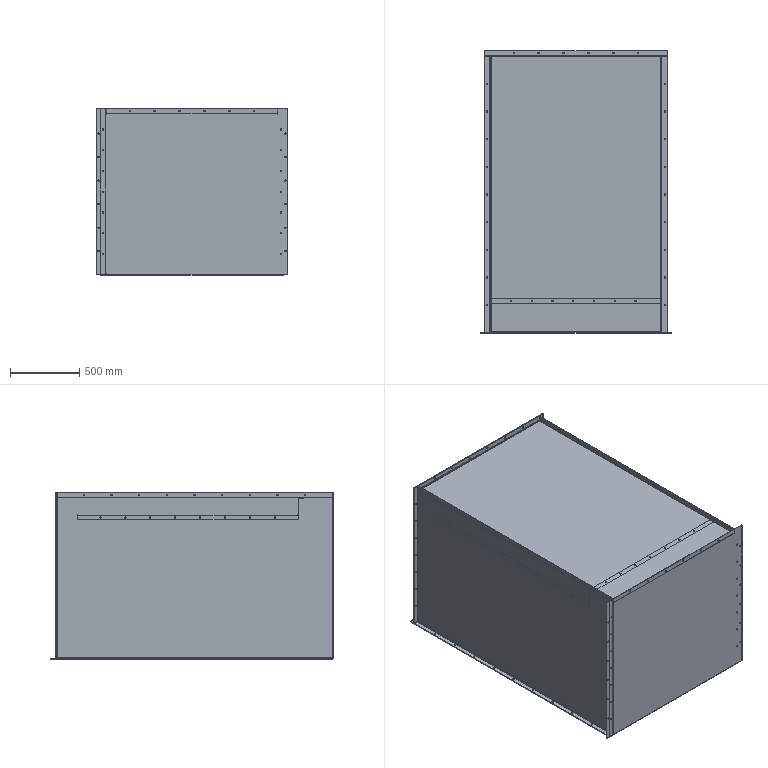Part | SolidWorks | 7 solids | 500 faces | box 1380 x 2043 x 1204 mm | volume 43462479 mm3 | cylinder 386 | plane 98 | spline 16 | commonest cylinder face diameters 10 x362 6 x12 12 x12